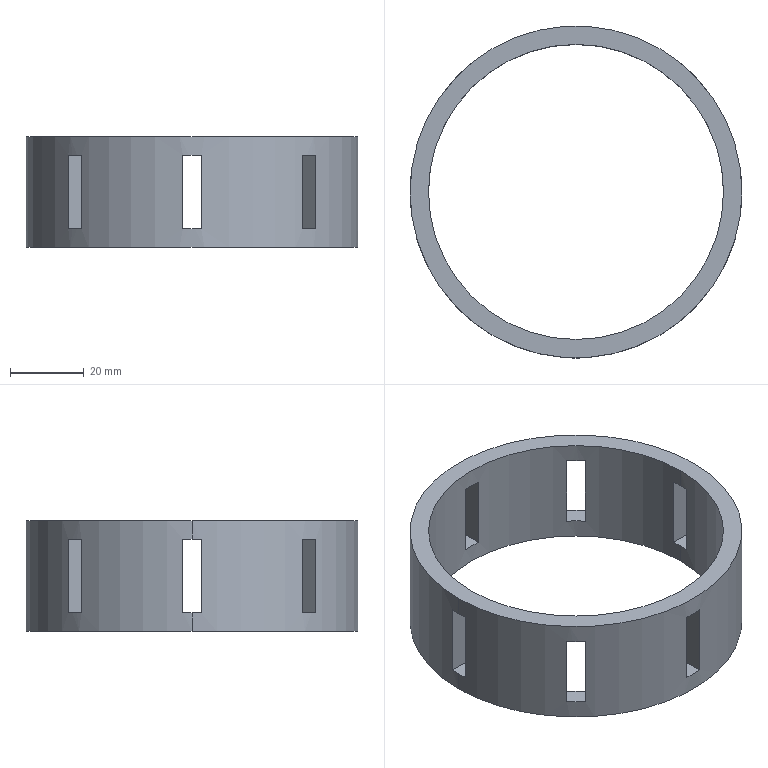Part | SolidWorks | features CirPattern 1, Cut 1, Extrusion 1 | 1 solid | 38 faces | box 90 x 90 x 30 mm | volume 36053 mm3 | plane 34 | cylinder 4 | commonest cylinder face diameters 80 x2 90 x2
STEP:
#1=CARTESIAN_POINT('',(-597.384,-129.922,25.));
#2=VERTEX_POINT('',#1);
#3=CARTESIAN_POINT('',(-597.384,-129.922,5.));
#4=VERTEX_POINT('',#3);
#5=CARTESIAN_POINT('',(-597.384,-129.922,30.));
#6=DIRECTION('',(0.,0.,-1.));
#7=VECTOR('',#6,1000.);
#8=LINE('',#5,#7);
#9=EDGE_CURVE('',#2,#4,#8,.T.);
#10=ORIENTED_EDGE('',*,*,#9,.F.);
#11=CARTESIAN_POINT('',(-602.384,-129.922,25.));
#12=VERTEX_POINT('',#11);
#13=CARTESIAN_POINT('',(-599.884,-90.,25.));
#14=DIRECTION('',(0.,0.,1.));
#15=DIRECTION('',(1.,0.,0.));
#16=AXIS2_PLACEMENT_3D('',#13,#14,#15);
#17=CIRCLE('',#16,40.);
#18=EDGE_CURVE('',#12,#2,#17,.T.);
#19=ORIENTED_EDGE('',*,*,#18,.F.);
#20=CARTESIAN_POINT('',(-602.384,-129.922,5.));
#21=VERTEX_POINT('',#20);
#22=CARTESIAN_POINT('',(-602.384,-129.922,30.));
#23=DIRECTION('',(0.,0.,1.));
#24=VECTOR('',#23,1000.);
#25=LINE('',#22,#24);
#26=EDGE_CURVE('',#21,#12,#25,.T.);
#27=ORIENTED_EDGE('',*,*,#26,.F.);
#28=CARTESIAN_POINT('',(-599.884,-90.,5.));
#29=DIRECTION('',(0.,0.,-1.));
#30=DIRECTION('',(-1.,0.,0.));
#31=AXIS2_PLACEMENT_3D('',#28,#29,#30);
#32=CIRCLE('',#31,40.);
#33=EDGE_CURVE('',#4,#21,#32,.T.);
#34=ORIENTED_EDGE('',*,*,#33,.F.);
#35=EDGE_LOOP('',(#10,#19,#27,#34));
#36=FACE_BOUND('',#35,.T.);
#37=CARTESIAN_POINT('',(-629.881,-116.461,5.));
#38=VERTEX_POINT('',#37);
#39=CARTESIAN_POINT('',(-629.881,-116.461,25.));
#40=VERTEX_POINT('',#39);
#41=CARTESIAN_POINT('',(-629.881,-116.461,30.));
#42=DIRECTION('',(0.,0.,1.));
#43=VECTOR('',#42,1000.);
#44=LINE('',#41,#43);
#45=EDGE_CURVE('',#38,#40,#44,.T.);
#46=ORIENTED_EDGE('',*,*,#45,.F.);
#47=CARTESIAN_POINT('',(-626.345,-119.997,5.));
#48=VERTEX_POINT('',#47);
#49=CARTESIAN_POINT('',(-599.884,-90.,5.));
#50=DIRECTION('',(0.,0.,-1.));
#51=DIRECTION('',(-1.,0.,0.));
#52=AXIS2_PLACEMENT_3D('',#49,#50,#51);
#53=CIRCLE('',#52,40.);
#54=EDGE_CURVE('',#48,#38,#53,.T.);
#55=ORIENTED_EDGE('',*,*,#54,.F.);
#56=CARTESIAN_POINT('',(-626.345,-119.997,25.));
#57=VERTEX_POINT('',#56);
#58=CARTESIAN_POINT('',(-626.345,-119.997,30.));
#59=DIRECTION('',(0.,0.,-1.));
#60=VECTOR('',#59,1000.);
#61=LINE('',#58,#60);
#62=EDGE_CURVE('',#57,#48,#61,.T.);
#63=ORIENTED_EDGE('',*,*,#62,.F.);
#64=CARTESIAN_POINT('',(-599.884,-90.,25.));
#65=DIRECTION('',(0.,0.,1.));
#66=DIRECTION('',(1.,0.,0.));
#67=AXIS2_PLACEMENT_3D('',#64,#65,#66);
#68=CIRCLE('',#67,40.);
#69=EDGE_CURVE('',#40,#57,#68,.T.);
#70=ORIENTED_EDGE('',*,*,#69,.F.);
#71=EDGE_LOOP('',(#46,#55,#63,#70));
#72=FACE_BOUND('',#71,.T.);
#73=CARTESIAN_POINT('',(-569.887,-116.461,25.));
#74=VERTEX_POINT('',#73);
#75=CARTESIAN_POINT('',(-569.887,-116.461,5.));
#76=VERTEX_POINT('',#75);
#77=CARTESIAN_POINT('',(-569.887,-116.461,30.));
#78=DIRECTION('',(0.,0.,-1.));
#79=VECTOR('',#78,1000.);
#80=LINE('',#77,#79);
#81=EDGE_CURVE('',#74,#76,#80,.T.);
#82=ORIENTED_EDGE('',*,*,#81,.F.);
#83=CARTESIAN_POINT('',(-573.423,-119.997,25.));
#84=VERTEX_POINT('',#83);
#85=CARTESIAN_POINT('',(-599.884,-90.,25.));
#86=DIRECTION('',(0.,0.,1.));
#87=DIRECTION('',(1.,0.,0.));
#88=AXIS2_PLACEMENT_3D('',#85,#86,#87);
#89=CIRCLE('',#88,40.);
#90=EDGE_CURVE('',#84,#74,#89,.T.);
#91=ORIENTED_EDGE('',*,*,#90,.F.);
#92=CARTESIAN_POINT('',(-573.423,-119.997,5.));
#93=VERTEX_POINT('',#92);
#94=CARTESIAN_POINT('',(-573.423,-119.997,30.));
#95=DIRECTION('',(0.,0.,1.));
#96=VECTOR('',#95,1000.);
#97=LINE('',#94,#96);
#98=EDGE_CURVE('',#93,#84,#97,.T.);
#99=ORIENTED_EDGE('',*,*,#98,.F.);
#100=CARTESIAN_POINT('',(-599.884,-90.,5.));
#101=DIRECTION('',(0.,0.,-1.));
#102=DIRECTION('',(-1.,0.,0.));
#103=AXIS2_PLACEMENT_3D('',#100,#101,#102);
#104=CIRCLE('',#103,40.);
#105=EDGE_CURVE('',#76,#93,#104,.T.);
#106=ORIENTED_EDGE('',*,*,#105,.F.);
#107=EDGE_LOOP('',(#82,#91,#99,#106));
#108=FACE_BOUND('',#107,.T.);
#109=CARTESIAN_POINT('',(-639.884,-90.,30.));
#110=VERTEX_POINT('',#109);
#111=CARTESIAN_POINT('',(-559.884,-90.,30.));
#112=VERTEX_POINT('',#111);
#113=CARTESIAN_POINT('',(-599.884,-90.,30.));
#114=DIRECTION('',(0.,0.,1.));
#115=DIRECTION('',(1.,0.,0.));
#116=AXIS2_PLACEMENT_3D('',#113,#114,#115);
#117=CIRCLE('',#116,40.);
#118=EDGE_CURVE('',#110,#112,#117,.T.);
#119=ORIENTED_EDGE('',*,*,#118,.T.);
#120=CARTESIAN_POINT('',(-559.884,-90.,25.));
#121=VERTEX_POINT('',#120);
#122=CARTESIAN_POINT('',(-559.884,-90.,30.));
#123=DIRECTION('',(0.,0.,-1.));
#124=VECTOR('',#123,1000.);
#125=LINE('',#122,#124);
#126=EDGE_CURVE('',#112,#121,#125,.T.);
#127=ORIENTED_EDGE('',*,*,#126,.T.);
#128=CARTESIAN_POINT('',(-559.962,-92.5,25.));
#129=VERTEX_POINT('',#128);
#130=CARTESIAN_POINT('',(-599.884,-90.,25.));
#131=DIRECTION('',(0.,0.,1.));
#132=DIRECTION('',(1.,0.,0.));
#133=AXIS2_PLACEMENT_3D('',#130,#131,#132);
#134=CIRCLE('',#133,40.);
#135=EDGE_CURVE('',#129,#121,#134,.T.);
#136=ORIENTED_EDGE('',*,*,#135,.F.);
#137=CARTESIAN_POINT('',(-559.962,-92.5,5.));
#138=VERTEX_POINT('',#137);
#139=CARTESIAN_POINT('',(-559.962,-92.5,30.));
#140=DIRECTION('',(0.,0.,1.));
#141=VECTOR('',#140,1000.);
#142=LINE('',#139,#141);
#143=EDGE_CURVE('',#138,#129,#142,.T.);
#144=ORIENTED_EDGE('',*,*,#143,.F.);
#145=CARTESIAN_POINT('',(-559.884,-90.,5.));
#146=VERTEX_POINT('',#145);
#147=CARTESIAN_POINT('',(-599.884,-90.,5.));
#148=DIRECTION('',(0.,0.,-1.));
#149=DIRECTION('',(-1.,0.,0.));
#150=AXIS2_PLACEMENT_3D('',#147,#148,#149);
#151=CIRCLE('',#150,40.);
#152=EDGE_CURVE('',#146,#138,#151,.T.);
#153=ORIENTED_EDGE('',*,*,#152,.F.);
#154=CARTESIAN_POINT('',(-559.884,-90.,0.));
#155=VERTEX_POINT('',#154);
#156=CARTESIAN_POINT('',(-559.884,-90.,30.));
#157=DIRECTION('',(0.,0.,-1.));
#158=VECTOR('',#157,1000.);
#159=LINE('',#156,#158);
#160=EDGE_CURVE('',#146,#155,#159,.T.);
#161=ORIENTED_EDGE('',*,*,#160,.T.);
#162=CARTESIAN_POINT('',(-639.884,-90.,0.));
#163=VERTEX_POINT('',#162);
#164=CARTESIAN_POINT('',(-599.884,-90.,0.));
#165=DIRECTION('',(0.,0.,1.));
#166=DIRECTION('',(1.,0.,0.));
#167=AXIS2_PLACEMENT_3D('',#164,#165,#166);
#168=CIRCLE('',#167,40.);
#169=EDGE_CURVE('',#163,#155,#168,.T.);
#170=ORIENTED_EDGE('',*,*,#169,.F.);
#171=CARTESIAN_POINT('',(-639.884,-90.,5.));
#172=VERTEX_POINT('',#171);
#173=CARTESIAN_POINT('',(-639.884,-90.,30.));
#174=DIRECTION('',(0.,0.,-1.));
#175=VECTOR('',#174,1000.);
#176=LINE('',#173,#175);
#177=EDGE_CURVE('',#172,#163,#176,.T.);
#178=ORIENTED_EDGE('',*,*,#177,.F.);
#179=CARTESIAN_POINT('',(-639.806,-92.5,5.));
#180=VERTEX_POINT('',#179);
#181=CARTESIAN_POINT('',(-599.884,-90.,5.));
#182=DIRECTION('',(0.,0.,-1.));
#183=DIRECTION('',(-1.,0.,0.));
#184=AXIS2_PLACEMENT_3D('',#181,#182,#183);
#185=CIRCLE('',#184,40.);
#186=EDGE_CURVE('',#180,#172,#185,.T.);
#187=ORIENTED_EDGE('',*,*,#186,.F.);
#188=CARTESIAN_POINT('',(-639.806,-92.5,25.));
#189=VERTEX_POINT('',#188);
#190=CARTESIAN_POINT('',(-639.806,-92.5,30.));
#191=DIRECTION('',(0.,0.,-1.));
#192=VECTOR('',#191,1000.);
#193=LINE('',#190,#192);
#194=EDGE_CURVE('',#189,#180,#193,.T.);
#195=ORIENTED_EDGE('',*,*,#194,.F.);
#196=CARTESIAN_POINT('',(-639.884,-90.,25.));
#197=VERTEX_POINT('',#196);
#198=CARTESIAN_POINT('',(-599.884,-90.,25.));
#199=DIRECTION('',(0.,0.,1.));
#200=DIRECTION('',(1.,0.,0.));
#201=AXIS2_PLACEMENT_3D('',#198,#199,#200);
#202=CIRCLE('',#201,40.);
#203=EDGE_CURVE('',#197,#189,#202,.T.);
#204=ORIENTED_EDGE('',*,*,#203,.F.);
#205=CARTESIAN_POINT('',(-639.884,-90.,30.));
#206=DIRECTION('',(0.,0.,-1.));
#207=VECTOR('',#206,1000.);
#208=LINE('',#205,#207);
#209=EDGE_CURVE('',#110,#197,#208,.T.);
#210=ORIENTED_EDGE('',*,*,#209,.F.);
#211=EDGE_LOOP('',(#119,#127,#136,#144,#153,#161,#170,#178,#187,#195,#204,#210));
#212=FACE_OUTER_BOUND('',#211,.T.);
#213=CARTESIAN_POINT('',(-599.884,-90.,30.));
#214=DIRECTION('',(0.,0.,-1.));
#215=DIRECTION('',(-1.,0.,0.));
#216=AXIS2_PLACEMENT_3D('',#213,#214,#215);
#217=CYLINDRICAL_SURFACE('',#216,40.);
#218=ADVANCED_FACE('',(#36,#72,#108,#212),#217,.F.);
#219=CARTESIAN_POINT('',(-602.384,-45.069,5.));
#220=VERTEX_POINT('',#219);
#221=CARTESIAN_POINT('',(-597.384,-45.069,5.));
#222=VERTEX_POINT('',#221);
#223=CARTESIAN_POINT('',(-599.884,-90.,5.));
#224=DIRECTION('',(0.,0.,-1.));
#225=DIRECTION('',(-1.,0.,0.));
#226=AXIS2_PLACEMENT_3D('',#223,#224,#225);
#227=CIRCLE('',#226,45.);
#228=EDGE_CURVE('',#220,#222,#227,.T.);
#229=ORIENTED_EDGE('',*,*,#228,.T.);
#230=CARTESIAN_POINT('',(-597.384,-45.069,25.));
#231=VERTEX_POINT('',#230);
#232=CARTESIAN_POINT('',(-597.384,-45.069,30.));
#233=DIRECTION('',(0.,0.,1.));
#234=VECTOR('',#233,1000.);
#235=LINE('',#232,#234);
#236=EDGE_CURVE('',#222,#231,#235,.T.);
#237=ORIENTED_EDGE('',*,*,#236,.T.);
#238=CARTESIAN_POINT('',(-602.384,-45.069,25.));
#239=VERTEX_POINT('',#238);
#240=CARTESIAN_POINT('',(-599.884,-90.,25.));
#241=DIRECTION('',(0.,0.,1.));
#242=DIRECTION('',(1.,0.,0.));
#243=AXIS2_PLACEMENT_3D('',#240,#241,#242);
#244=CIRCLE('',#243,45.);
#245=EDGE_CURVE('',#231,#239,#244,.T.);
#246=ORIENTED_EDGE('',*,*,#245,.T.);
#247=CARTESIAN_POINT('',(-602.384,-45.069,30.));
#248=DIRECTION('',(0.,0.,-1.));
#249=VECTOR('',#248,1000.);
#250=LINE('',#247,#249);
#251=EDGE_CURVE('',#239,#220,#250,.T.);
#252=ORIENTED_EDGE('',*,*,#251,.T.);
#253=EDGE_LOOP('',(#229,#237,#246,#252));
#254=FACE_BOUND('',#253,.T.);
#255=CARTESIAN_POINT('',(-566.346,-59.997,25.));
#256=VERTEX_POINT('',#255);
#257=CARTESIAN_POINT('',(-569.881,-56.462,25.));
#258=VERTEX_POINT('',#257);
#259=CARTESIAN_POINT('',(-599.884,-90.,25.));
#260=DIRECTION('',(0.,0.,1.));
#261=DIRECTION('',(1.,0.,0.));
#262=AXIS2_PLACEMENT_3D('',#259,#260,#261);
#263=CIRCLE('',#262,45.);
#264=EDGE_CURVE('',#256,#258,#263,.T.);
#265=ORIENTED_EDGE('',*,*,#264,.T.);
#266=CARTESIAN_POINT('',(-569.881,-56.462,5.));
#267=VERTEX_POINT('',#266);
#268=CARTESIAN_POINT('',(-569.881,-56.462,30.));
#269=DIRECTION('',(0.,0.,-1.));
#270=VECTOR('',#269,1000.);
#271=LINE('',#268,#270);
#272=EDGE_CURVE('',#258,#267,#271,.T.);
#273=ORIENTED_EDGE('',*,*,#272,.T.);
#274=CARTESIAN_POINT('',(-566.346,-59.997,5.));
#275=VERTEX_POINT('',#274);
#276=CARTESIAN_POINT('',(-599.884,-90.,5.));
#277=DIRECTION('',(0.,0.,-1.));
#278=DIRECTION('',(-1.,0.,0.));
#279=AXIS2_PLACEMENT_3D('',#276,#277,#278);
#280=CIRCLE('',#279,45.);
#281=EDGE_CURVE('',#267,#275,#280,.T.);
#282=ORIENTED_EDGE('',*,*,#281,.T.);
#283=CARTESIAN_POINT('',(-566.346,-59.997,30.));
#284=DIRECTION('',(0.,0.,1.));
#285=VECTOR('',#284,1000.);
#286=LINE('',#283,#285);
#287=EDGE_CURVE('',#275,#256,#286,.T.);
#288=ORIENTED_EDGE('',*,*,#287,.T.);
#289=EDGE_LOOP('',(#265,#273,#282,#288));
#290=FACE_BOUND('',#289,.T.);
#291=CARTESIAN_POINT('',(-629.887,-56.462,5.));
#292=VERTEX_POINT('',#291);
#293=CARTESIAN_POINT('',(-629.887,-56.462,25.));
#294=VERTEX_POINT('',#293);
#295=CARTESIAN_POINT('',(-629.887,-56.462,30.));
#296=DIRECTION('',(0.,0.,1.));
#297=VECTOR('',#296,1000.);
#298=LINE('',#295,#297);
#299=EDGE_CURVE('',#292,#294,#298,.T.);
#300=ORIENTED_EDGE('',*,*,#299,.T.);
#301=CARTESIAN_POINT('',(-633.423,-59.997,25.));
#302=VERTEX_POINT('',#301);
#303=CARTESIAN_POINT('',(-599.884,-90.,25.));
#304=DIRECTION('',(0.,0.,1.));
#305=DIRECTION('',(1.,0.,0.));
#306=AXIS2_PLACEMENT_3D('',#303,#304,#305);
#307=CIRCLE('',#306,45.);
#308=EDGE_CURVE('',#294,#302,#307,.T.);
#309=ORIENTED_EDGE('',*,*,#308,.T.);
#310=CARTESIAN_POINT('',(-633.423,-59.997,5.));
#311=VERTEX_POINT('',#310);
#312=CARTESIAN_POINT('',(-633.423,-59.997,30.));
#313=DIRECTION('',(0.,0.,-1.));
#314=VECTOR('',#313,1000.);
#315=LINE('',#312,#314);
#316=EDGE_CURVE('',#302,#311,#315,.T.);
#317=ORIENTED_EDGE('',*,*,#316,.T.);
#318=CARTESIAN_POINT('',(-599.884,-90.,5.));
#319=DIRECTION('',(0.,0.,-1.));
#320=DIRECTION('',(-1.,0.,0.));
#321=AXIS2_PLACEMENT_3D('',#318,#319,#320);
#322=CIRCLE('',#321,45.);
#323=EDGE_CURVE('',#311,#292,#322,.T.);
#324=ORIENTED_EDGE('',*,*,#323,.T.);
#325=EDGE_LOOP('',(#300,#309,#317,#324));
#326=FACE_BOUND('',#325,.T.);
#327=CARTESIAN_POINT('',(-554.884,-90.,30.));
#328=VERTEX_POINT('',#327);
#329=CARTESIAN_POINT('',(-644.884,-90.,30.));
#330=VERTEX_POINT('',#329);
#331=CARTESIAN_POINT('',(-599.884,-90.,30.));
#332=DIRECTION('',(0.,0.,1.));
#333=DIRECTION('',(1.,0.,0.));
#334=AXIS2_PLACEMENT_3D('',#331,#332,#333);
#335=CIRCLE('',#334,45.);
#336=EDGE_CURVE('',#328,#330,#335,.T.);
#337=ORIENTED_EDGE('',*,*,#336,.F.);
#338=CARTESIAN_POINT('',(-554.884,-90.,25.));
#339=VERTEX_POINT('',#338);
#340=CARTESIAN_POINT('',(-554.884,-90.,30.));
#341=DIRECTION('',(0.,0.,-1.));
#342=VECTOR('',#341,1000.);
#343=LINE('',#340,#342);
#344=EDGE_CURVE('',#328,#339,#343,.T.);
#345=ORIENTED_EDGE('',*,*,#344,.T.);
#346=CARTESIAN_POINT('',(-554.954,-87.5,25.));
#347=VERTEX_POINT('',#346);
#348=CARTESIAN_POINT('',(-599.884,-90.,25.));
#349=DIRECTION('',(0.,0.,1.));
#350=DIRECTION('',(1.,0.,0.));
#351=AXIS2_PLACEMENT_3D('',#348,#349,#350);
#352=CIRCLE('',#351,45.);
#353=EDGE_CURVE('',#339,#347,#352,.T.);
#354=ORIENTED_EDGE('',*,*,#353,.T.);
#355=CARTESIAN_POINT('',(-554.954,-87.5,5.));
#356=VERTEX_POINT('',#355);
#357=CARTESIAN_POINT('',(-554.954,-87.5,30.));
#358=DIRECTION('',(0.,0.,-1.));
#359=VECTOR('',#358,1000.);
#360=LINE('',#357,#359);
#361=EDGE_CURVE('',#347,#356,#360,.T.);
#362=ORIENTED_EDGE('',*,*,#361,.T.);
#363=CARTESIAN_POINT('',(-554.884,-90.,5.));
#364=VERTEX_POINT('',#363);
#365=CARTESIAN_POINT('',(-599.884,-90.,5.));
#366=DIRECTION('',(0.,0.,-1.));
#367=DIRECTION('',(-1.,0.,0.));
#368=AXIS2_PLACEMENT_3D('',#365,#366,#367);
#369=CIRCLE('',#368,45.);
#370=EDGE_CURVE('',#356,#364,#369,.T.);
#371=ORIENTED_EDGE('',*,*,#370,.T.);
#372=CARTESIAN_POINT('',(-554.884,-90.,0.));
#373=VERTEX_POINT('',#372);
#374=CARTESIAN_POINT('',(-554.884,-90.,30.));
#375=DIRECTION('',(0.,0.,-1.));
#376=VECTOR('',#375,1000.);
#377=LINE('',#374,#376);
#378=EDGE_CURVE('',#364,#373,#377,.T.);
#379=ORIENTED_EDGE('',*,*,#378,.T.);
#380=CARTESIAN_POINT('',(-644.884,-90.,0.));
#381=VERTEX_POINT('',#380);
#382=CARTESIAN_POINT('',(-599.884,-90.,0.));
#383=DIRECTION('',(0.,0.,1.));
#384=DIRECTION('',(1.,0.,0.));
#385=AXIS2_PLACEMENT_3D('',#382,#383,#384);
#386=CIRCLE('',#385,45.);
#387=EDGE_CURVE('',#373,#381,#386,.T.);
#388=ORIENTED_EDGE('',*,*,#387,.T.);
#389=CARTESIAN_POINT('',(-644.884,-90.,5.));
#390=VERTEX_POINT('',#389);
#391=CARTESIAN_POINT('',(-644.884,-90.,30.));
#392=DIRECTION('',(0.,0.,-1.));
#393=VECTOR('',#392,1000.);
#394=LINE('',#391,#393);
#395=EDGE_CURVE('',#390,#381,#394,.T.);
#396=ORIENTED_EDGE('',*,*,#395,.F.);
#397=CARTESIAN_POINT('',(-644.815,-87.5,5.));
#398=VERTEX_POINT('',#397);
#399=CARTESIAN_POINT('',(-599.884,-90.,5.));
#400=DIRECTION('',(0.,0.,-1.));
#401=DIRECTION('',(-1.,0.,0.));
#402=AXIS2_PLACEMENT_3D('',#399,#400,#401);
#403=CIRCLE('',#402,45.);
#404=EDGE_CURVE('',#390,#398,#403,.T.);
#405=ORIENTED_EDGE('',*,*,#404,.T.);
#406=CARTESIAN_POINT('',(-644.815,-87.5,25.));
#407=VERTEX_POINT('',#406);
#408=CARTESIAN_POINT('',(-644.815,-87.5,30.));
#409=DIRECTION('',(0.,0.,1.));
#410=VECTOR('',#409,1000.);
#411=LINE('',#408,#410);
#412=EDGE_CURVE('',#398,#407,#411,.T.);
#413=ORIENTED_EDGE('',*,*,#412,.T.);
#414=CARTESIAN_POINT('',(-644.884,-90.,25.));
#415=VERTEX_POINT('',#414);
#416=CARTESIAN_POINT('',(-599.884,-90.,25.));
#417=DIRECTION('',(0.,0.,1.));
#418=DIRECTION('',(1.,0.,0.));
#419=AXIS2_PLACEMENT_3D('',#416,#417,#418);
#420=CIRCLE('',#419,45.);
#421=EDGE_CURVE('',#407,#415,#420,.T.);
#422=ORIENTED_EDGE('',*,*,#421,.T.);
#423=CARTESIAN_POINT('',(-644.884,-90.,30.));
#424=DIRECTION('',(0.,0.,-1.));
#425=VECTOR('',#424,1000.);
#426=LINE('',#423,#425);
#427=EDGE_CURVE('',#330,#415,#426,.T.);
#428=ORIENTED_EDGE('',*,*,#427,.F.);
#429=EDGE_LOOP('',(#337,#345,#354,#362,#371,#379,#388,#396,#405,#413,#422,#428));
#430=FACE_OUTER_BOUND('',#429,.T.);
#431=CARTESIAN_POINT('',(-599.884,-90.,30.));
#432=DIRECTION('',(0.,0.,-1.));
#433=DIRECTION('',(-1.,0.,0.));
#434=AXIS2_PLACEMENT_3D('',#431,#432,#433);
#435=CYLINDRICAL_SURFACE('',#434,45.);
#436=ADVANCED_FACE('',(#254,#290,#326,#430),#435,.T.);
#437=CARTESIAN_POINT('',(-599.884,-90.,30.));
#438=DIRECTION('',(0.,0.,1.));
#439=DIRECTION('',(1.,0.,0.));
#440=AXIS2_PLACEMENT_3D('',#437,#438,#439);
#441=CIRCLE('',#440,45.);
#442=EDGE_CURVE('',#330,#328,#441,.T.);
#443=ORIENTED_EDGE('',*,*,#442,.T.);
#444=ORIENTED_EDGE('',*,*,#336,.T.);
#445=EDGE_LOOP('',(#443,#444));
#446=FACE_OUTER_BOUND('',#445,.T.);
#447=ORIENTED_EDGE('',*,*,#118,.F.);
#448=CARTESIAN_POINT('',(-599.884,-90.,30.));
#449=DIRECTION('',(0.,0.,1.));
#450=DIRECTION('',(1.,0.,0.));
#451=AXIS2_PLACEMENT_3D('',#448,#449,#450);
#452=CIRCLE('',#451,40.);
#453=EDGE_CURVE('',#112,#110,#452,.T.);
#454=ORIENTED_EDGE('',*,*,#453,.F.);
#455=EDGE_LOOP('',(#447,#454));
#456=FACE_BOUND('',#455,.T.);
#457=CARTESIAN_POINT('',(-599.884,-90.,30.));
#458=DIRECTION('',(0.,0.,1.));
#459=DIRECTION('',(1.,0.,0.));
#460=AXIS2_PLACEMENT_3D('',#457,#458,#459);
#461=PLANE('',#460);
#462=ADVANCED_FACE('',(#446,#456),#461,.T.);
#463=CARTESIAN_POINT('',(-599.884,-90.,0.));
#464=DIRECTION('',(0.,0.,1.));
#465=DIRECTION('',(1.,0.,0.));
#466=AXIS2_PLACEMENT_3D('',#463,#464,#465);
#467=CIRCLE('',#466,45.);
#468=EDGE_CURVE('',#381,#373,#467,.T.);
#469=ORIENTED_EDGE('',*,*,#468,.F.);
#470=ORIENTED_EDGE('',*,*,#387,.F.);
#471=EDGE_LOOP('',(#469,#470));
#472=FACE_OUTER_BOUND('',#471,.T.);
#473=ORIENTED_EDGE('',*,*,#169,.T.);
#474=CARTESIAN_POINT('',(-599.884,-90.,0.));
#475=DIRECTION('',(0.,0.,1.));
#476=DIRECTION('',(1.,0.,0.));
#477=AXIS2_PLACEMENT_3D('',#474,#475,#476);
#478=CIRCLE('',#477,40.);
#479=EDGE_CURVE('',#155,#163,#478,.T.);
#480=ORIENTED_EDGE('',*,*,#479,.T.);
#481=EDGE_LOOP('',(#473,#480));
#482=FACE_BOUND('',#481,.T.);
#483=CARTESIAN_POINT('',(-599.884,-90.,0.));
#484=DIRECTION('',(0.,0.,1.));
#485=DIRECTION('',(1.,0.,0.));
#486=AXIS2_PLACEMENT_3D('',#483,#484,#485);
#487=PLANE('',#486);
#488=ADVANCED_FACE('',(#472,#482),#487,.F.);
#489=ORIENTED_EDGE('',*,*,#344,.F.);
#490=ORIENTED_EDGE('',*,*,#442,.F.);
#491=ORIENTED_EDGE('',*,*,#427,.T.);
#492=CARTESIAN_POINT('',(-644.815,-92.5,25.));
#493=VERTEX_POINT('',#492);
#494=CARTESIAN_POINT('',(-599.884,-90.,25.));
#495=DIRECTION('',(0.,0.,1.));
#496=DIRECTION('',(1.,0.,0.));
#497=AXIS2_PLACEMENT_3D('',#494,#495,#496);
#498=CIRCLE('',#497,45.);
#499=EDGE_CURVE('',#415,#493,#498,.T.);
#500=ORIENTED_EDGE('',*,*,#499,.T.);
#501=CARTESIAN_POINT('',(-644.815,-92.5,5.));
#502=VERTEX_POINT('',#501);
#503=CARTESIAN_POINT('',(-644.815,-92.5,30.));
#504=DIRECTION('',(0.,0.,-1.));
#505=VECTOR('',#504,1000.);
#506=LINE('',#503,#505);
#507=EDGE_CURVE('',#493,#502,#506,.T.);
#508=ORIENTED_EDGE('',*,*,#507,.T.);
#509=CARTESIAN_POINT('',(-599.884,-90.,5.));
#510=DIRECTION('',(0.,0.,-1.));
#511=DIRECTION('',(-1.,0.,0.));
#512=AXIS2_PLACEMENT_3D('',#509,#510,#511);
#513=CIRCLE('',#512,45.);
#514=EDGE_CURVE('',#502,#390,#513,.T.);
#515=ORIENTED_EDGE('',*,*,#514,.T.);
#516=ORIENTED_EDGE('',*,*,#395,.T.);
#517=ORIENTED_EDGE('',*,*,#468,.T.);
#518=ORIENTED_EDGE('',*,*,#378,.F.);
#519=CARTESIAN_POINT('',(-554.954,-92.5,5.));
#520=VERTEX_POINT('',#519);
#521=CARTESIAN_POINT('',(-599.884,-90.,5.));
#522=DIRECTION('',(0.,0.,-1.));
#523=DIRECTION('',(-1.,0.,0.));
#524=AXIS2_PLACEMENT_3D('',#521,#522,#523);
#525=CIRCLE('',#524,45.);
#526=EDGE_CURVE('',#364,#520,#525,.T.);
#527=ORIENTED_EDGE('',*,*,#526,.T.);
#528=CARTESIAN_POINT('',(-554.954,-92.5,25.));
#529=VERTEX_POINT('',#528);
#530=CARTESIAN_POINT('',(-554.954,-92.5,30.));
#531=DIRECTION('',(0.,0.,1.));
#532=VECTOR('',#531,1000.);
#533=LINE('',#530,#532);
#534=EDGE_CURVE('',#520,#529,#533,.T.);
#535=ORIENTED_EDGE('',*,*,#534,.T.);
#536=CARTESIAN_POINT('',(-599.884,-90.,25.));
#537=DIRECTION('',(0.,0.,1.));
#538=DIRECTION('',(1.,0.,0.));
#539=AXIS2_PLACEMENT_3D('',#536,#537,#538);
#540=CIRCLE('',#539,45.);
#541=EDGE_CURVE('',#529,#339,#540,.T.);
#542=ORIENTED_EDGE('',*,*,#541,.T.);
#543=EDGE_LOOP('',(#489,#490,#491,#500,#508,#515,#516,#517,#518,#527,#535,#542));
#544=FACE_OUTER_BOUND('',#543,.T.);
#545=CARTESIAN_POINT('',(-569.881,-123.538,25.));
#546=VERTEX_POINT('',#545);
#547=CARTESIAN_POINT('',(-566.346,-120.003,25.));
#548=VERTEX_POINT('',#547);
#549=CARTESIAN_POINT('',(-599.884,-90.,25.));
#550=DIRECTION('',(0.,0.,1.));
#551=DIRECTION('',(1.,0.,0.));
#552=AXIS2_PLACEMENT_3D('',#549,#550,#551);
#553=CIRCLE('',#552,45.);
#554=EDGE_CURVE('',#546,#548,#553,.T.);
#555=ORIENTED_EDGE('',*,*,#554,.T.);
#556=CARTESIAN_POINT('',(-566.346,-120.003,5.));
#557=VERTEX_POINT('',#556);
#558=CARTESIAN_POINT('',(-566.346,-120.003,30.));
#559=DIRECTION('',(0.,0.,-1.));
#560=VECTOR('',#559,1000.);
#561=LINE('',#558,#560);
#562=EDGE_CURVE('',#548,#557,#561,.T.);
#563=ORIENTED_EDGE('',*,*,#562,.T.);
#564=CARTESIAN_POINT('',(-569.881,-123.538,5.));
#565=VERTEX_POINT('',#564);
#566=CARTESIAN_POINT('',(-599.884,-90.,5.));
#567=DIRECTION('',(0.,0.,-1.));
#568=DIRECTION('',(-1.,0.,0.));
#569=AXIS2_PLACEMENT_3D('',#566,#567,#568);
#570=CIRCLE('',#569,45.);
#571=EDGE_CURVE('',#557,#565,#570,.T.);
#572=ORIENTED_EDGE('',*,*,#571,.T.);
#573=CARTESIAN_POINT('',(-569.881,-123.538,30.));
#574=DIRECTION('',(0.,0.,1.));
#575=VECTOR('',#574,1000.);
#576=LINE('',#573,#575);
#577=EDGE_CURVE('',#565,#546,#576,.T.);
#578=ORIENTED_EDGE('',*,*,#577,.T.);
#579=EDGE_LOOP('',(#555,#563,#572,#578));
#580=FACE_BOUND('',#579,.T.);
#581=CARTESIAN_POINT('',(-629.887,-123.538,5.));
#582=VERTEX_POINT('',#581);
#583=CARTESIAN_POINT('',(-633.423,-120.003,5.));
#584=VERTEX_POINT('',#583);
#585=CARTESIAN_POINT('',(-599.884,-90.,5.));
#586=DIRECTION('',(0.,0.,-1.));
#587=DIRECTION('',(-1.,0.,0.));
#588=AXIS2_PLACEMENT_3D('',#585,#586,#587);
#589=CIRCLE('',#588,45.);
#590=EDGE_CURVE('',#582,#584,#589,.T.);
#591=ORIENTED_EDGE('',*,*,#590,.T.);
#592=CARTESIAN_POINT('',(-633.423,-120.003,25.));
#593=VERTEX_POINT('',#592);
#594=CARTESIAN_POINT('',(-633.423,-120.003,30.));
#595=DIRECTION('',(0.,0.,1.));
#596=VECTOR('',#595,1000.);
#597=LINE('',#594,#596);
#598=EDGE_CURVE('',#584,#593,#597,.T.);
#599=ORIENTED_EDGE('',*,*,#598,.T.);
#600=CARTESIAN_POINT('',(-629.887,-123.538,25.));
#601=VERTEX_POINT('',#600);
#602=CARTESIAN_POINT('',(-599.884,-90.,25.));
#603=DIRECTION('',(0.,0.,1.));
#604=DIRECTION('',(1.,0.,0.));
#605=AXIS2_PLACEMENT_3D('',#602,#603,#604);
#606=CIRCLE('',#605,45.);
#607=EDGE_CURVE('',#593,#601,#606,.T.);
#608=ORIENTED_EDGE('',*,*,#607,.T.);
#609=CARTESIAN_POINT('',(-629.887,-123.538,30.));
#610=DIRECTION('',(0.,0.,-1.));
#611=VECTOR('',#610,1000.);
#612=LINE('',#609,#611);
#613=EDGE_CURVE('',#601,#582,#612,.T.);
#614=ORIENTED_EDGE('',*,*,#613,.T.);
#615=EDGE_LOOP('',(#591,#599,#608,#614));
#616=FACE_BOUND('',#615,.T.);
#617=CARTESIAN_POINT('',(-597.384,-134.931,25.));
#618=VERTEX_POINT('',#617);
#619=CARTESIAN_POINT('',(-597.384,-134.931,5.));
#620=VERTEX_POINT('',#619);
#621=CARTESIAN_POINT('',(-597.384,-134.931,30.));
#622=DIRECTION('',(0.,0.,-1.));
#623=VECTOR('',#622,1000.);
#624=LINE('',#621,#623);
#625=EDGE_CURVE('',#618,#620,#624,.T.);
#626=ORIENTED_EDGE('',*,*,#625,.T.);
#627=CARTESIAN_POINT('',(-602.384,-134.931,5.));
#628=VERTEX_POINT('',#627);
#629=CARTESIAN_POINT('',(-599.884,-90.,5.));
#630=DIRECTION('',(0.,0.,-1.));
#631=DIRECTION('',(-1.,0.,0.));
#632=AXIS2_PLACEMENT_3D('',#629,#630,#631);
#633=CIRCLE('',#632,45.);
#634=EDGE_CURVE('',#620,#628,#633,.T.);
#635=ORIENTED_EDGE('',*,*,#634,.T.);
#636=CARTESIAN_POINT('',(-602.384,-134.931,25.));
#637=VERTEX_POINT('',#636);
#638=CARTESIAN_POINT('',(-602.384,-134.931,30.));
#639=DIRECTION('',(0.,0.,1.));
#640=VECTOR('',#639,1000.);
#641=LINE('',#638,#640);
#642=EDGE_CURVE('',#628,#637,#641,.T.);
#643=ORIENTED_EDGE('',*,*,#642,.T.);
#644=CARTESIAN_POINT('',(-599.884,-90.,25.));
#645=DIRECTION('',(0.,0.,1.));
#646=DIRECTION('',(1.,0.,0.));
#647=AXIS2_PLACEMENT_3D('',#644,#645,#646);
#648=CIRCLE('',#647,45.);
#649=EDGE_CURVE('',#637,#618,#648,.T.);
#650=ORIENTED_EDGE('',*,*,#649,.T.);
#651=EDGE_LOOP('',(#626,#635,#643,#650));
#652=FACE_BOUND('',#651,.T.);
#653=CARTESIAN_POINT('',(-599.884,-90.,30.));
#654=DIRECTION('',(0.,0.,-1.));
#655=DIRECTION('',(-1.,0.,0.));
#656=AXIS2_PLACEMENT_3D('',#653,#654,#655);
#657=CYLINDRICAL_SURFACE('',#656,45.);
#658=ADVANCED_FACE('',(#544,#580,#616,#652),#657,.T.);
#659=ORIENTED_EDGE('',*,*,#126,.F.);
#660=ORIENTED_EDGE('',*,*,#453,.T.);
#661=ORIENTED_EDGE('',*,*,#209,.T.);
#662=CARTESIAN_POINT('',(-639.806,-87.5,25.));
#663=VERTEX_POINT('',#662);
#664=CARTESIAN_POINT('',(-599.884,-90.,25.));
#665=DIRECTION('',(0.,0.,1.));
#666=DIRECTION('',(1.,0.,0.));
#667=AXIS2_PLACEMENT_3D('',#664,#665,#666);
#668=CIRCLE('',#667,40.);
#669=EDGE_CURVE('',#663,#197,#668,.T.);
#670=ORIENTED_EDGE('',*,*,#669,.F.);
#671=CARTESIAN_POINT('',(-639.806,-87.5,5.));
#672=VERTEX_POINT('',#671);
#673=CARTESIAN_POINT('',(-639.806,-87.5,30.));
#674=DIRECTION('',(0.,0.,1.));
#675=VECTOR('',#674,1000.);
#676=LINE('',#673,#675);
#677=EDGE_CURVE('',#672,#663,#676,.T.);
#678=ORIENTED_EDGE('',*,*,#677,.F.);
#679=CARTESIAN_POINT('',(-599.884,-90.,5.));
#680=DIRECTION('',(0.,0.,-1.));
#681=DIRECTION('',(-1.,0.,0.));
#682=AXIS2_PLACEMENT_3D('',#679,#680,#681);
#683=CIRCLE('',#682,40.);
#684=EDGE_CURVE('',#172,#672,#683,.T.);
#685=ORIENTED_EDGE('',*,*,#684,.F.);
#686=ORIENTED_EDGE('',*,*,#177,.T.);
#687=ORIENTED_EDGE('',*,*,#479,.F.);
#688=ORIENTED_EDGE('',*,*,#160,.F.);
#689=CARTESIAN_POINT('',(-559.962,-87.5,5.));
#690=VERTEX_POINT('',#689);
#691=CARTESIAN_POINT('',(-599.884,-90.,5.));
#692=DIRECTION('',(0.,0.,-1.));
#693=DIRECTION('',(-1.,0.,0.));
#694=AXIS2_PLACEMENT_3D('',#691,#692,#693);
#695=CIRCLE('',#694,40.);
#696=EDGE_CURVE('',#690,#146,#695,.T.);
#697=ORIENTED_EDGE('',*,*,#696,.F.);
#698=CARTESIAN_POINT('',(-559.962,-87.5,25.));
#699=VERTEX_POINT('',#698);
#700=CARTESIAN_POINT('',(-559.962,-87.5,30.));
#701=DIRECTION('',(0.,0.,-1.));
#702=VECTOR('',#701,1000.);
#703=LINE('',#700,#702);
#704=EDGE_CURVE('',#699,#690,#703,.T.);
#705=ORIENTED_EDGE('',*,*,#704,.F.);
#706=CARTESIAN_POINT('',(-599.884,-90.,25.));
#707=DIRECTION('',(0.,0.,1.));
#708=DIRECTION('',(1.,0.,0.));
#709=AXIS2_PLACEMENT_3D('',#706,#707,#708);
#710=CIRCLE('',#709,40.);
#711=EDGE_CURVE('',#121,#699,#710,.T.);
#712=ORIENTED_EDGE('',*,*,#711,.F.);
#713=EDGE_LOOP('',(#659,#660,#661,#670,#678,#685,#686,#687,#688,#697,#705,#712));
#714=FACE_OUTER_BOUND('',#713,.T.);
#715=CARTESIAN_POINT('',(-626.345,-60.003,25.));
#716=VERTEX_POINT('',#715);
#717=CARTESIAN_POINT('',(-629.881,-63.539,25.));
#718=VERTEX_POINT('',#717);
#719=CARTESIAN_POINT('',(-599.884,-90.,25.));
#720=DIRECTION('',(0.,0.,1.));
#721=DIRECTION('',(1.,0.,0.));
#722=AXIS2_PLACEMENT_3D('',#719,#720,#721);
#723=CIRCLE('',#722,40.);
#724=EDGE_CURVE('',#716,#718,#723,.T.);
#725=ORIENTED_EDGE('',*,*,#724,.F.);
#726=CARTESIAN_POINT('',(-626.345,-60.003,5.));
#727=VERTEX_POINT('',#726);
#728=CARTESIAN_POINT('',(-626.345,-60.003,30.));
#729=DIRECTION('',(0.,0.,1.));
#730=VECTOR('',#729,1000.);
#731=LINE('',#728,#730);
#732=EDGE_CURVE('',#727,#716,#731,.T.);
#733=ORIENTED_EDGE('',*,*,#732,.F.);
#734=CARTESIAN_POINT('',(-629.881,-63.539,5.));
#735=VERTEX_POINT('',#734);
#736=CARTESIAN_POINT('',(-599.884,-90.,5.));
#737=DIRECTION('',(0.,0.,-1.));
#738=DIRECTION('',(-1.,0.,0.));
#739=AXIS2_PLACEMENT_3D('',#736,#737,#738);
#740=CIRCLE('',#739,40.);
#741=EDGE_CURVE('',#735,#727,#740,.T.);
#742=ORIENTED_EDGE('',*,*,#741,.F.);
#743=CARTESIAN_POINT('',(-629.881,-63.539,30.));
#744=DIRECTION('',(0.,0.,-1.));
#745=VECTOR('',#744,1000.);
#746=LINE('',#743,#745);
#747=EDGE_CURVE('',#718,#735,#746,.T.);
#748=ORIENTED_EDGE('',*,*,#747,.F.);
#749=EDGE_LOOP('',(#725,#733,#742,#748));
#750=FACE_BOUND('',#749,.T.);
#751=CARTESIAN_POINT('',(-573.423,-60.003,25.));
#752=VERTEX_POINT('',#751);
#753=CARTESIAN_POINT('',(-573.423,-60.003,5.));
#754=VERTEX_POINT('',#753);
#755=CARTESIAN_POINT('',(-573.423,-60.003,30.));
#756=DIRECTION('',(0.,0.,-1.));
#757=VECTOR('',#756,1000.);
#758=LINE('',#755,#757);
#759=EDGE_CURVE('',#752,#754,#758,.T.);
#760=ORIENTED_EDGE('',*,*,#759,.F.);
#761=CARTESIAN_POINT('',(-569.887,-63.539,25.));
#762=VERTEX_POINT('',#761);
#763=CARTESIAN_POINT('',(-599.884,-90.,25.));
#764=DIRECTION('',(0.,0.,1.));
#765=DIRECTION('',(1.,0.,0.));
#766=AXIS2_PLACEMENT_3D('',#763,#764,#765);
#767=CIRCLE('',#766,40.);
#768=EDGE_CURVE('',#762,#752,#767,.T.);
#769=ORIENTED_EDGE('',*,*,#768,.F.);
#770=CARTESIAN_POINT('',(-569.887,-63.539,5.));
#771=VERTEX_POINT('',#770);
#772=CARTESIAN_POINT('',(-569.887,-63.539,30.));
#773=DIRECTION('',(0.,0.,1.));
#774=VECTOR('',#773,1000.);
#775=LINE('',#772,#774);
#776=EDGE_CURVE('',#771,#762,#775,.T.);
#777=ORIENTED_EDGE('',*,*,#776,.F.);
#778=CARTESIAN_POINT('',(-599.884,-90.,5.));
#779=DIRECTION('',(0.,0.,-1.));
#780=DIRECTION('',(-1.,0.,0.));
#781=AXIS2_PLACEMENT_3D('',#778,#779,#780);
#782=CIRCLE('',#781,40.);
#783=EDGE_CURVE('',#754,#771,#782,.T.);
#784=ORIENTED_EDGE('',*,*,#783,.F.);
#785=EDGE_LOOP('',(#760,#769,#777,#784));
#786=FACE_BOUND('',#785,.T.);
#787=CARTESIAN_POINT('',(-597.384,-50.078,5.));
#788=VERTEX_POINT('',#787);
#789=CARTESIAN_POINT('',(-597.384,-50.078,25.));
#790=VERTEX_POINT('',#789);
#791=CARTESIAN_POINT('',(-597.384,-50.078,30.));
#792=DIRECTION('',(0.,0.,1.));
#793=VECTOR('',#792,1000.);
#794=LINE('',#791,#793);
#795=EDGE_CURVE('',#788,#790,#794,.T.);
#796=ORIENTED_EDGE('',*,*,#795,.F.);
#797=CARTESIAN_POINT('',(-602.384,-50.078,5.));
#798=VERTEX_POINT('',#797);
#799=CARTESIAN_POINT('',(-599.884,-90.,5.));
#800=DIRECTION('',(0.,0.,-1.));
#801=DIRECTION('',(-1.,0.,0.));
#802=AXIS2_PLACEMENT_3D('',#799,#800,#801);
#803=CIRCLE('',#802,40.);
#804=EDGE_CURVE('',#798,#788,#803,.T.);
#805=ORIENTED_EDGE('',*,*,#804,.F.);
#806=CARTESIAN_POINT('',(-602.384,-50.078,25.));
#807=VERTEX_POINT('',#806);
#808=CARTESIAN_POINT('',(-602.384,-50.078,30.));
#809=DIRECTION('',(0.,0.,-1.));
#810=VECTOR('',#809,1000.);
#811=LINE('',#808,#810);
#812=EDGE_CURVE('',#807,#798,#811,.T.);
#813=ORIENTED_EDGE('',*,*,#812,.F.);
#814=CARTESIAN_POINT('',(-599.884,-90.,25.));
#815=DIRECTION('',(0.,0.,1.));
#816=DIRECTION('',(1.,0.,0.));
#817=AXIS2_PLACEMENT_3D('',#814,#815,#816);
#818=CIRCLE('',#817,40.);
#819=EDGE_CURVE('',#790,#807,#818,.T.);
#820=ORIENTED_EDGE('',*,*,#819,.F.);
#821=EDGE_LOOP('',(#796,#805,#813,#820));
#822=FACE_BOUND('',#821,.T.);
#823=CARTESIAN_POINT('',(-599.884,-90.,30.));
#824=DIRECTION('',(0.,0.,-1.));
#825=DIRECTION('',(-1.,0.,0.));
#826=AXIS2_PLACEMENT_3D('',#823,#824,#825);
#827=CYLINDRICAL_SURFACE('',#826,40.);
#828=ADVANCED_FACE('',(#714,#750,#786,#822),#827,.F.);
#829=CARTESIAN_POINT('',(-597.384,-135.,5.));
#830=DIRECTION('',(0.,1.,0.));
#831=VECTOR('',#830,1000.);
#832=LINE('',#829,#831);
#833=EDGE_CURVE('',#620,#4,#832,.T.);
#834=ORIENTED_EDGE('',*,*,#833,.T.);
#835=ORIENTED_EDGE('',*,*,#33,.T.);
#836=CARTESIAN_POINT('',(-602.384,-135.,5.));
#837=DIRECTION('',(0.,1.,0.));
#838=VECTOR('',#837,1000.);
#839=LINE('',#836,#838);
#840=EDGE_CURVE('',#628,#21,#839,.T.);
#841=ORIENTED_EDGE('',*,*,#840,.F.);
#842=ORIENTED_EDGE('',*,*,#634,.F.);
#843=EDGE_LOOP('',(#834,#835,#841,#842));
#844=FACE_OUTER_BOUND('',#843,.T.);
#845=CARTESIAN_POINT('',(-602.384,-135.,5.));
#846=DIRECTION('',(0.,0.,-1.));
#847=DIRECTION('',(-1.,0.,0.));
#848=AXIS2_PLACEMENT_3D('',#845,#846,#847);
#849=PLANE('',#848);
#850=ADVANCED_FACE('',(#844),#849,.F.);
#851=ORIENTED_EDGE('',*,*,#840,.T.);
#852=ORIENTED_EDGE('',*,*,#26,.T.);
#853=CARTESIAN_POINT('',(-602.384,-135.,25.));
#854=DIRECTION('',(0.,1.,0.));
#855=VECTOR('',#854,1000.);
#856=LINE('',#853,#855);
#857=EDGE_CURVE('',#637,#12,#856,.T.);
#858=ORIENTED_EDGE('',*,*,#857,.F.);
#859=ORIENTED_EDGE('',*,*,#642,.F.);
#860=EDGE_LOOP('',(#851,#852,#858,#859));
#861=FACE_OUTER_BOUND('',#860,.T.);
#862=CARTESIAN_POINT('',(-602.384,-135.,25.));
#863=DIRECTION('',(-1.,0.,0.));
#864=DIRECTION('',(0.,0.,1.));
#865=AXIS2_PLACEMENT_3D('',#862,#863,#864);
#866=PLANE('',#865);
#867=ADVANCED_FACE('',(#861),#866,.F.);
#868=ORIENTED_EDGE('',*,*,#857,.T.);
#869=ORIENTED_EDGE('',*,*,#18,.T.);
#870=CARTESIAN_POINT('',(-597.384,-135.,25.));
#871=DIRECTION('',(0.,1.,0.));
#872=VECTOR('',#871,1000.);
#873=LINE('',#870,#872);
#874=EDGE_CURVE('',#618,#2,#873,.T.);
#875=ORIENTED_EDGE('',*,*,#874,.F.);
#876=ORIENTED_EDGE('',*,*,#649,.F.);
#877=EDGE_LOOP('',(#868,#869,#875,#876));
#878=FACE_OUTER_BOUND('',#877,.T.);
#879=CARTESIAN_POINT('',(-602.384,-135.,25.));
#880=DIRECTION('',(0.,0.,1.));
#881=DIRECTION('',(1.,0.,0.));
#882=AXIS2_PLACEMENT_3D('',#879,#880,#881);
#883=PLANE('',#882);
#884=ADVANCED_FACE('',(#878),#883,.F.);
#885=ORIENTED_EDGE('',*,*,#874,.T.);
#886=ORIENTED_EDGE('',*,*,#9,.T.);
#887=ORIENTED_EDGE('',*,*,#833,.F.);
#888=ORIENTED_EDGE('',*,*,#625,.F.);
#889=EDGE_LOOP('',(#885,#886,#887,#888));
#890=FACE_OUTER_BOUND('',#889,.T.);
#891=CARTESIAN_POINT('',(-597.384,-135.,25.));
#892=DIRECTION('',(1.,0.,0.));
#893=DIRECTION('',(0.,0.,-1.));
#894=AXIS2_PLACEMENT_3D('',#891,#892,#893);
#895=PLANE('',#894);
#896=ADVANCED_FACE('',(#890),#895,.F.);
#897=CARTESIAN_POINT('',(-597.384,-135.,5.));
#898=DIRECTION('',(0.,1.,0.));
#899=VECTOR('',#898,1000.);
#900=LINE('',#897,#899);
#901=EDGE_CURVE('',#788,#222,#900,.T.);
#902=ORIENTED_EDGE('',*,*,#901,.F.);
#903=ORIENTED_EDGE('',*,*,#795,.T.);
#904=CARTESIAN_POINT('',(-597.384,-135.,25.));
#905=DIRECTION('',(0.,1.,0.));
#906=VECTOR('',#905,1000.);
#907=LINE('',#904,#906);
#908=EDGE_CURVE('',#790,#231,#907,.T.);
#909=ORIENTED_EDGE('',*,*,#908,.T.);
#910=ORIENTED_EDGE('',*,*,#236,.F.);
#911=EDGE_LOOP('',(#902,#903,#909,#910));
#912=FACE_OUTER_BOUND('',#911,.T.);
#913=CARTESIAN_POINT('',(-597.384,-135.,25.));
#914=DIRECTION('',(1.,0.,0.));
#915=DIRECTION('',(0.,0.,-1.));
#916=AXIS2_PLACEMENT_3D('',#913,#914,#915);
#917=PLANE('',#916);
#918=ADVANCED_FACE('',(#912),#917,.F.);
#919=ORIENTED_EDGE('',*,*,#908,.F.);
#920=ORIENTED_EDGE('',*,*,#819,.T.);
#921=CARTESIAN_POINT('',(-602.384,-135.,25.));
#922=DIRECTION('',(0.,1.,0.));
#923=VECTOR('',#922,1000.);
#924=LINE('',#921,#923);
#925=EDGE_CURVE('',#807,#239,#924,.T.);
#926=ORIENTED_EDGE('',*,*,#925,.T.);
#927=ORIENTED_EDGE('',*,*,#245,.F.);
#928=EDGE_LOOP('',(#919,#920,#926,#927));
#929=FACE_OUTER_BOUND('',#928,.T.);
#930=CARTESIAN_POINT('',(-602.384,-135.,25.));
#931=DIRECTION('',(0.,0.,1.));
#932=DIRECTION('',(1.,0.,0.));
#933=AXIS2_PLACEMENT_3D('',#930,#931,#932);
#934=PLANE('',#933);
#935=ADVANCED_FACE('',(#929),#934,.F.);
#936=ORIENTED_EDGE('',*,*,#925,.F.);
#937=ORIENTED_EDGE('',*,*,#812,.T.);
#938=CARTESIAN_POINT('',(-602.384,-135.,5.));
#939=DIRECTION('',(0.,1.,0.));
#940=VECTOR('',#939,1000.);
#941=LINE('',#938,#940);
#942=EDGE_CURVE('',#798,#220,#941,.T.);
#943=ORIENTED_EDGE('',*,*,#942,.T.);
#944=ORIENTED_EDGE('',*,*,#251,.F.);
#945=EDGE_LOOP('',(#936,#937,#943,#944));
#946=FACE_OUTER_BOUND('',#945,.T.);
#947=CARTESIAN_POINT('',(-602.384,-135.,25.));
#948=DIRECTION('',(-1.,0.,0.));
#949=DIRECTION('',(0.,0.,1.));
#950=AXIS2_PLACEMENT_3D('',#947,#948,#949);
#951=PLANE('',#950);
#952=ADVANCED_FACE('',(#946),#951,.F.);
#953=ORIENTED_EDGE('',*,*,#942,.F.);
#954=ORIENTED_EDGE('',*,*,#804,.T.);
#955=ORIENTED_EDGE('',*,*,#901,.T.);
#956=ORIENTED_EDGE('',*,*,#228,.F.);
#957=EDGE_LOOP('',(#953,#954,#955,#956));
#958=FACE_OUTER_BOUND('',#957,.T.);
#959=CARTESIAN_POINT('',(-602.384,-135.,5.));
#960=DIRECTION('',(0.,0.,-1.));
#961=DIRECTION('',(-1.,0.,0.));
#962=AXIS2_PLACEMENT_3D('',#959,#960,#961);
#963=PLANE('',#962);
#964=ADVANCED_FACE('',(#958),#963,.F.);
#965=CARTESIAN_POINT('',(-553.116,-46.768,5.));
#966=DIRECTION('',(-0.7071,-0.7071,0.));
#967=VECTOR('',#966,1000.);
#968=LINE('',#965,#967);
#969=EDGE_CURVE('',#275,#771,#968,.T.);
#970=ORIENTED_EDGE('',*,*,#969,.T.);
#971=ORIENTED_EDGE('',*,*,#776,.T.);
#972=CARTESIAN_POINT('',(-553.116,-46.768,25.));
#973=DIRECTION('',(-0.7071,-0.7071,0.));
#974=VECTOR('',#973,1000.);
#975=LINE('',#972,#974);
#976=EDGE_CURVE('',#256,#762,#975,.T.);
#977=ORIENTED_EDGE('',*,*,#976,.F.);
#978=ORIENTED_EDGE('',*,*,#287,.F.);
#979=EDGE_LOOP('',(#970,#971,#977,#978));
#980=FACE_OUTER_BOUND('',#979,.T.);
#981=CARTESIAN_POINT('',(-553.116,-46.768,25.));
#982=DIRECTION('',(0.7071,-0.7071,0.));
#983=DIRECTION('',(0.7071,0.7071,0.));
#984=AXIS2_PLACEMENT_3D('',#981,#982,#983);
#985=PLANE('',#984);
#986=ADVANCED_FACE('',(#980),#985,.F.);
#987=CARTESIAN_POINT('',(-556.652,-43.232,25.));
#988=DIRECTION('',(-0.7071,-0.7071,0.));
#989=VECTOR('',#988,1000.);
#990=LINE('',#987,#989);
#991=EDGE_CURVE('',#258,#752,#990,.T.);
#992=ORIENTED_EDGE('',*,*,#991,.T.);
#993=ORIENTED_EDGE('',*,*,#759,.T.);
#994=CARTESIAN_POINT('',(-556.652,-43.232,5.));
#995=DIRECTION('',(-0.7071,-0.7071,0.));
#996=VECTOR('',#995,1000.);
#997=LINE('',#994,#996);
#998=EDGE_CURVE('',#267,#754,#997,.T.);
#999=ORIENTED_EDGE('',*,*,#998,.F.);
#1000=ORIENTED_EDGE('',*,*,#272,.F.);
#1001=EDGE_LOOP('',(#992,#993,#999,#1000));
#1002=FACE_OUTER_BOUND('',#1001,.T.);
#1003=CARTESIAN_POINT('',(-556.652,-43.232,25.));
#1004=DIRECTION('',(-0.7071,0.7071,0.));
#1005=DIRECTION('',(-0.7071,-0.7071,0.));
#1006=AXIS2_PLACEMENT_3D('',#1003,#1004,#1005);
#1007=PLANE('',#1006);
#1008=ADVANCED_FACE('',(#1002),#1007,.F.);
#1009=ORIENTED_EDGE('',*,*,#998,.T.);
#1010=ORIENTED_EDGE('',*,*,#783,.T.);
#1011=ORIENTED_EDGE('',*,*,#969,.F.);
#1012=ORIENTED_EDGE('',*,*,#281,.F.);
#1013=EDGE_LOOP('',(#1009,#1010,#1011,#1012));
#1014=FACE_OUTER_BOUND('',#1013,.T.);
#1015=CARTESIAN_POINT('',(-556.652,-136.768,5.));
#1016=DIRECTION('',(0.,0.,-1.));
#1017=DIRECTION('',(-1.,0.,0.));
#1018=AXIS2_PLACEMENT_3D('',#1015,#1016,#1017);
#1019=PLANE('',#1018);
#1020=ADVANCED_FACE('',(#1014),#1019,.F.);
#1021=ORIENTED_EDGE('',*,*,#976,.T.);
#1022=ORIENTED_EDGE('',*,*,#768,.T.);
#1023=ORIENTED_EDGE('',*,*,#991,.F.);
#1024=ORIENTED_EDGE('',*,*,#264,.F.);
#1025=EDGE_LOOP('',(#1021,#1022,#1023,#1024));
#1026=FACE_OUTER_BOUND('',#1025,.T.);
#1027=CARTESIAN_POINT('',(-556.652,-136.768,25.));
#1028=DIRECTION('',(0.,0.,1.));
#1029=DIRECTION('',(1.,0.,0.));
#1030=AXIS2_PLACEMENT_3D('',#1027,#1028,#1029);
#1031=PLANE('',#1030);
#1032=ADVANCED_FACE('',(#1026),#1031,.F.);
#1033=CARTESIAN_POINT('',(-554.884,-92.5,5.));
#1034=DIRECTION('',(-1.,0.,0.));
#1035=VECTOR('',#1034,1000.);
#1036=LINE('',#1033,#1035);
#1037=EDGE_CURVE('',#520,#138,#1036,.T.);
#1038=ORIENTED_EDGE('',*,*,#1037,.T.);
#1039=ORIENTED_EDGE('',*,*,#143,.T.);
#1040=CARTESIAN_POINT('',(-554.884,-92.5,25.));
#1041=DIRECTION('',(-1.,0.,0.));
#1042=VECTOR('',#1041,1000.);
#1043=LINE('',#1040,#1042);
#1044=EDGE_CURVE('',#529,#129,#1043,.T.);
#1045=ORIENTED_EDGE('',*,*,#1044,.F.);
#1046=ORIENTED_EDGE('',*,*,#534,.F.);
#1047=EDGE_LOOP('',(#1038,#1039,#1045,#1046));
#1048=FACE_OUTER_BOUND('',#1047,.T.);
#1049=CARTESIAN_POINT('',(-554.884,-92.5,25.));
#1050=DIRECTION('',(0.,-1.,0.));
#1051=DIRECTION('',(1.,0.,0.));
#1052=AXIS2_PLACEMENT_3D('',#1049,#1050,#1051);
#1053=PLANE('',#1052);
#1054=ADVANCED_FACE('',(#1048),#1053,.F.);
#1055=CARTESIAN_POINT('',(-554.884,-87.5,25.));
#1056=DIRECTION('',(-1.,0.,0.));
#1057=VECTOR('',#1056,1000.);
#1058=LINE('',#1055,#1057);
#1059=EDGE_CURVE('',#347,#699,#1058,.T.);
#1060=ORIENTED_EDGE('',*,*,#1059,.T.);
#1061=ORIENTED_EDGE('',*,*,#704,.T.);
#1062=CARTESIAN_POINT('',(-554.884,-87.5,5.));
#1063=DIRECTION('',(-1.,0.,0.));
#1064=VECTOR('',#1063,1000.);
#1065=LINE('',#1062,#1064);
#1066=EDGE_CURVE('',#356,#690,#1065,.T.);
#1067=ORIENTED_EDGE('',*,*,#1066,.F.);
#1068=ORIENTED_EDGE('',*,*,#361,.F.);
#1069=EDGE_LOOP('',(#1060,#1061,#1067,#1068));
#1070=FACE_OUTER_BOUND('',#1069,.T.);
#1071=CARTESIAN_POINT('',(-554.884,-87.5,25.));
#1072=DIRECTION('',(0.,1.,0.));
#1073=DIRECTION('',(-1.,0.,0.));
#1074=AXIS2_PLACEMENT_3D('',#1071,#1072,#1073);
#1075=PLANE('',#1074);
#1076=ADVANCED_FACE('',(#1070),#1075,.F.);
#1077=ORIENTED_EDGE('',*,*,#1066,.T.);
#1078=ORIENTED_EDGE('',*,*,#696,.T.);
#1079=ORIENTED_EDGE('',*,*,#152,.T.);
#1080=ORIENTED_EDGE('',*,*,#1037,.F.);
#1081=ORIENTED_EDGE('',*,*,#526,.F.);
#1082=ORIENTED_EDGE('',*,*,#370,.F.);
#1083=EDGE_LOOP('',(#1077,#1078,#1079,#1080,#1081,#1082));
#1084=FACE_OUTER_BOUND('',#1083,.T.);
#1085=CARTESIAN_POINT('',(-556.652,-136.768,5.));
#1086=DIRECTION('',(0.,0.,-1.));
#1087=DIRECTION('',(-1.,0.,0.));
#1088=AXIS2_PLACEMENT_3D('',#1085,#1086,#1087);
#1089=PLANE('',#1088);
#1090=ADVANCED_FACE('',(#1084),#1089,.F.);
#1091=ORIENTED_EDGE('',*,*,#1044,.T.);
#1092=ORIENTED_EDGE('',*,*,#135,.T.);
#1093=ORIENTED_EDGE('',*,*,#711,.T.);
#1094=ORIENTED_EDGE('',*,*,#1059,.F.);
#1095=ORIENTED_EDGE('',*,*,#353,.F.);
#1096=ORIENTED_EDGE('',*,*,#541,.F.);
#1097=EDGE_LOOP('',(#1091,#1092,#1093,#1094,#1095,#1096));
#1098=FACE_OUTER_BOUND('',#1097,.T.);
#1099=CARTESIAN_POINT('',(-556.652,-136.768,25.));
#1100=DIRECTION('',(0.,0.,1.));
#1101=DIRECTION('',(1.,0.,0.));
#1102=AXIS2_PLACEMENT_3D('',#1099,#1100,#1101);
#1103=PLANE('',#1102);
#1104=ADVANCED_FACE('',(#1098),#1103,.F.);
#1105=CARTESIAN_POINT('',(-554.884,-87.5,5.));
#1106=DIRECTION('',(-1.,0.,0.));
#1107=VECTOR('',#1106,1000.);
#1108=LINE('',#1105,#1107);
#1109=EDGE_CURVE('',#672,#398,#1108,.T.);
#1110=ORIENTED_EDGE('',*,*,#1109,.F.);
#1111=ORIENTED_EDGE('',*,*,#677,.T.);
#1112=CARTESIAN_POINT('',(-554.884,-87.5,25.));
#1113=DIRECTION('',(-1.,0.,0.));
#1114=VECTOR('',#1113,1000.);
#1115=LINE('',#1112,#1114);
#1116=EDGE_CURVE('',#663,#407,#1115,.T.);
#1117=ORIENTED_EDGE('',*,*,#1116,.T.);
#1118=ORIENTED_EDGE('',*,*,#412,.F.);
#1119=EDGE_LOOP('',(#1110,#1111,#1117,#1118));
#1120=FACE_OUTER_BOUND('',#1119,.T.);
#1121=CARTESIAN_POINT('',(-554.884,-87.5,25.));
#1122=DIRECTION('',(0.,1.,0.));
#1123=DIRECTION('',(-1.,0.,0.));
#1124=AXIS2_PLACEMENT_3D('',#1121,#1122,#1123);
#1125=PLANE('',#1124);
#1126=ADVANCED_FACE('',(#1120),#1125,.F.);
#1127=CARTESIAN_POINT('',(-554.884,-92.5,25.));
#1128=DIRECTION('',(-1.,0.,0.));
#1129=VECTOR('',#1128,1000.);
#1130=LINE('',#1127,#1129);
#1131=EDGE_CURVE('',#189,#493,#1130,.T.);
#1132=ORIENTED_EDGE('',*,*,#1131,.F.);
#1133=ORIENTED_EDGE('',*,*,#194,.T.);
#1134=CARTESIAN_POINT('',(-554.884,-92.5,5.));
#1135=DIRECTION('',(-1.,0.,0.));
#1136=VECTOR('',#1135,1000.);
#1137=LINE('',#1134,#1136);
#1138=EDGE_CURVE('',#180,#502,#1137,.T.);
#1139=ORIENTED_EDGE('',*,*,#1138,.T.);
#1140=ORIENTED_EDGE('',*,*,#507,.F.);
#1141=EDGE_LOOP('',(#1132,#1133,#1139,#1140));
#1142=FACE_OUTER_BOUND('',#1141,.T.);
#1143=CARTESIAN_POINT('',(-554.884,-92.5,25.));
#1144=DIRECTION('',(0.,-1.,0.));
#1145=DIRECTION('',(1.,0.,0.));
#1146=AXIS2_PLACEMENT_3D('',#1143,#1144,#1145);
#1147=PLANE('',#1146);
#1148=ADVANCED_FACE('',(#1142),#1147,.F.);
#1149=ORIENTED_EDGE('',*,*,#1138,.F.);
#1150=ORIENTED_EDGE('',*,*,#186,.T.);
#1151=ORIENTED_EDGE('',*,*,#684,.T.);
#1152=ORIENTED_EDGE('',*,*,#1109,.T.);
#1153=ORIENTED_EDGE('',*,*,#404,.F.);
#1154=ORIENTED_EDGE('',*,*,#514,.F.);
#1155=EDGE_LOOP('',(#1149,#1150,#1151,#1152,#1153,#1154));
#1156=FACE_OUTER_BOUND('',#1155,.T.);
#1157=CARTESIAN_POINT('',(-556.652,-136.768,5.));
#1158=DIRECTION('',(0.,0.,-1.));
#1159=DIRECTION('',(-1.,0.,0.));
#1160=AXIS2_PLACEMENT_3D('',#1157,#1158,#1159);
#1161=PLANE('',#1160);
#1162=ADVANCED_FACE('',(#1156),#1161,.F.);
#1163=ORIENTED_EDGE('',*,*,#1116,.F.);
#1164=ORIENTED_EDGE('',*,*,#669,.T.);
#1165=ORIENTED_EDGE('',*,*,#203,.T.);
#1166=ORIENTED_EDGE('',*,*,#1131,.T.);
#1167=ORIENTED_EDGE('',*,*,#499,.F.);
#1168=ORIENTED_EDGE('',*,*,#421,.F.);
#1169=EDGE_LOOP('',(#1163,#1164,#1165,#1166,#1167,#1168));
#1170=FACE_OUTER_BOUND('',#1169,.T.);
#1171=CARTESIAN_POINT('',(-556.652,-136.768,25.));
#1172=DIRECTION('',(0.,0.,1.));
#1173=DIRECTION('',(1.,0.,0.));
#1174=AXIS2_PLACEMENT_3D('',#1171,#1172,#1173);
#1175=PLANE('',#1174);
#1176=ADVANCED_FACE('',(#1170),#1175,.F.);
#1177=CARTESIAN_POINT('',(-556.652,-43.232,5.));
#1178=DIRECTION('',(-0.7071,-0.7071,0.));
#1179=VECTOR('',#1178,1000.);
#1180=LINE('',#1177,#1179);
#1181=EDGE_CURVE('',#38,#584,#1180,.T.);
#1182=ORIENTED_EDGE('',*,*,#1181,.F.);
#1183=ORIENTED_EDGE('',*,*,#45,.T.);
#1184=CARTESIAN_POINT('',(-556.652,-43.232,25.));
#1185=DIRECTION('',(-0.7071,-0.7071,0.));
#1186=VECTOR('',#1185,1000.);
#1187=LINE('',#1184,#1186);
#1188=EDGE_CURVE('',#40,#593,#1187,.T.);
#1189=ORIENTED_EDGE('',*,*,#1188,.T.);
#1190=ORIENTED_EDGE('',*,*,#598,.F.);
#1191=EDGE_LOOP('',(#1182,#1183,#1189,#1190));
#1192=FACE_OUTER_BOUND('',#1191,.T.);
#1193=CARTESIAN_POINT('',(-556.652,-43.232,25.));
#1194=DIRECTION('',(-0.7071,0.7071,0.));
#1195=DIRECTION('',(-0.7071,-0.7071,0.));
#1196=AXIS2_PLACEMENT_3D('',#1193,#1194,#1195);
#1197=PLANE('',#1196);
#1198=ADVANCED_FACE('',(#1192),#1197,.F.);
#1199=CARTESIAN_POINT('',(-553.116,-46.768,25.));
#1200=DIRECTION('',(-0.7071,-0.7071,0.));
#1201=VECTOR('',#1200,1000.);
#1202=LINE('',#1199,#1201);
#1203=EDGE_CURVE('',#57,#601,#1202,.T.);
#1204=ORIENTED_EDGE('',*,*,#1203,.F.);
#1205=ORIENTED_EDGE('',*,*,#62,.T.);
#1206=CARTESIAN_POINT('',(-553.116,-46.768,5.));
#1207=DIRECTION('',(-0.7071,-0.7071,0.));
#1208=VECTOR('',#1207,1000.);
#1209=LINE('',#1206,#1208);
#1210=EDGE_CURVE('',#48,#582,#1209,.T.);
#1211=ORIENTED_EDGE('',*,*,#1210,.T.);
#1212=ORIENTED_EDGE('',*,*,#613,.F.);
#1213=EDGE_LOOP('',(#1204,#1205,#1211,#1212));
#1214=FACE_OUTER_BOUND('',#1213,.T.);
#1215=CARTESIAN_POINT('',(-553.116,-46.768,25.));
#1216=DIRECTION('',(0.7071,-0.7071,0.));
#1217=DIRECTION('',(0.7071,0.7071,0.));
#1218=AXIS2_PLACEMENT_3D('',#1215,#1216,#1217);
#1219=PLANE('',#1218);
#1220=ADVANCED_FACE('',(#1214),#1219,.F.);
#1221=ORIENTED_EDGE('',*,*,#1210,.F.);
#1222=ORIENTED_EDGE('',*,*,#54,.T.);
#1223=ORIENTED_EDGE('',*,*,#1181,.T.);
#1224=ORIENTED_EDGE('',*,*,#590,.F.);
#1225=EDGE_LOOP('',(#1221,#1222,#1223,#1224));
#1226=FACE_OUTER_BOUND('',#1225,.T.);
#1227=CARTESIAN_POINT('',(-556.652,-136.768,5.));
#1228=DIRECTION('',(0.,0.,-1.));
#1229=DIRECTION('',(-1.,0.,0.));
#1230=AXIS2_PLACEMENT_3D('',#1227,#1228,#1229);
#1231=PLANE('',#1230);
#1232=ADVANCED_FACE('',(#1226),#1231,.F.);
#1233=ORIENTED_EDGE('',*,*,#1188,.F.);
#1234=ORIENTED_EDGE('',*,*,#69,.T.);
#1235=ORIENTED_EDGE('',*,*,#1203,.T.);
#1236=ORIENTED_EDGE('',*,*,#607,.F.);
#1237=EDGE_LOOP('',(#1233,#1234,#1235,#1236));
#1238=FACE_OUTER_BOUND('',#1237,.T.);
#1239=CARTESIAN_POINT('',(-556.652,-136.768,25.));
#1240=DIRECTION('',(0.,0.,1.));
#1241=DIRECTION('',(1.,0.,0.));
#1242=AXIS2_PLACEMENT_3D('',#1239,#1240,#1241);
#1243=PLANE('',#1242);
#1244=ADVANCED_FACE('',(#1238),#1243,.F.);
#1245=CARTESIAN_POINT('',(-553.116,-133.232,5.));
#1246=DIRECTION('',(-0.7071,0.7071,0.));
#1247=VECTOR('',#1246,1000.);
#1248=LINE('',#1245,#1247);
#1249=EDGE_CURVE('',#557,#76,#1248,.T.);
#1250=ORIENTED_EDGE('',*,*,#1249,.T.);
#1251=ORIENTED_EDGE('',*,*,#105,.T.);
#1252=CARTESIAN_POINT('',(-556.652,-136.768,5.));
#1253=DIRECTION('',(-0.7071,0.7071,0.));
#1254=VECTOR('',#1253,1000.);
#1255=LINE('',#1252,#1254);
#1256=EDGE_CURVE('',#565,#93,#1255,.T.);
#1257=ORIENTED_EDGE('',*,*,#1256,.F.);
#1258=ORIENTED_EDGE('',*,*,#571,.F.);
#1259=EDGE_LOOP('',(#1250,#1251,#1257,#1258));
#1260=FACE_OUTER_BOUND('',#1259,.T.);
#1261=CARTESIAN_POINT('',(-556.652,-136.768,5.));
#1262=DIRECTION('',(0.,0.,-1.));
#1263=DIRECTION('',(-1.,0.,0.));
#1264=AXIS2_PLACEMENT_3D('',#1261,#1262,#1263);
#1265=PLANE('',#1264);
#1266=ADVANCED_FACE('',(#1260),#1265,.F.);
#1267=ORIENTED_EDGE('',*,*,#1256,.T.);
#1268=ORIENTED_EDGE('',*,*,#98,.T.);
#1269=CARTESIAN_POINT('',(-556.652,-136.768,25.));
#1270=DIRECTION('',(-0.7071,0.7071,0.));
#1271=VECTOR('',#1270,1000.);
#1272=LINE('',#1269,#1271);
#1273=EDGE_CURVE('',#546,#84,#1272,.T.);
#1274=ORIENTED_EDGE('',*,*,#1273,.F.);
#1275=ORIENTED_EDGE('',*,*,#577,.F.);
#1276=EDGE_LOOP('',(#1267,#1268,#1274,#1275));
#1277=FACE_OUTER_BOUND('',#1276,.T.);
#1278=CARTESIAN_POINT('',(-556.652,-136.768,25.));
#1279=DIRECTION('',(-0.7071,-0.7071,0.));
#1280=DIRECTION('',(0.7071,-0.7071,0.));
#1281=AXIS2_PLACEMENT_3D('',#1278,#1279,#1280);
#1282=PLANE('',#1281);
#1283=ADVANCED_FACE('',(#1277),#1282,.F.);
#1284=ORIENTED_EDGE('',*,*,#1273,.T.);
#1285=ORIENTED_EDGE('',*,*,#90,.T.);
#1286=CARTESIAN_POINT('',(-553.116,-133.232,25.));
#1287=DIRECTION('',(-0.7071,0.7071,0.));
#1288=VECTOR('',#1287,1000.);
#1289=LINE('',#1286,#1288);
#1290=EDGE_CURVE('',#548,#74,#1289,.T.);
#1291=ORIENTED_EDGE('',*,*,#1290,.F.);
#1292=ORIENTED_EDGE('',*,*,#554,.F.);
#1293=EDGE_LOOP('',(#1284,#1285,#1291,#1292));
#1294=FACE_OUTER_BOUND('',#1293,.T.);
#1295=CARTESIAN_POINT('',(-556.652,-136.768,25.));
#1296=DIRECTION('',(0.,0.,1.));
#1297=DIRECTION('',(1.,0.,0.));
#1298=AXIS2_PLACEMENT_3D('',#1295,#1296,#1297);
#1299=PLANE('',#1298);
#1300=ADVANCED_FACE('',(#1294),#1299,.F.);
#1301=ORIENTED_EDGE('',*,*,#1290,.T.);
#1302=ORIENTED_EDGE('',*,*,#81,.T.);
#1303=ORIENTED_EDGE('',*,*,#1249,.F.);
#1304=ORIENTED_EDGE('',*,*,#562,.F.);
#1305=EDGE_LOOP('',(#1301,#1302,#1303,#1304));
#1306=FACE_OUTER_BOUND('',#1305,.T.);
#1307=CARTESIAN_POINT('',(-553.116,-133.232,25.));
#1308=DIRECTION('',(0.7071,0.7071,0.));
#1309=DIRECTION('',(-0.7071,0.7071,0.));
#1310=AXIS2_PLACEMENT_3D('',#1307,#1308,#1309);
#1311=PLANE('',#1310);
#1312=ADVANCED_FACE('',(#1306),#1311,.F.);
#1313=CARTESIAN_POINT('',(-556.652,-136.768,25.));
#1314=DIRECTION('',(-0.7071,0.7071,0.));
#1315=VECTOR('',#1314,1000.);
#1316=LINE('',#1313,#1315);
#1317=EDGE_CURVE('',#718,#302,#1316,.T.);
#1318=ORIENTED_EDGE('',*,*,#1317,.F.);
#1319=ORIENTED_EDGE('',*,*,#747,.T.);
#1320=CARTESIAN_POINT('',(-556.652,-136.768,5.));
#1321=DIRECTION('',(-0.7071,0.7071,0.));
#1322=VECTOR('',#1321,1000.);
#1323=LINE('',#1320,#1322);
#1324=EDGE_CURVE('',#735,#311,#1323,.T.);
#1325=ORIENTED_EDGE('',*,*,#1324,.T.);
#1326=ORIENTED_EDGE('',*,*,#316,.F.);
#1327=EDGE_LOOP('',(#1318,#1319,#1325,#1326));
#1328=FACE_OUTER_BOUND('',#1327,.T.);
#1329=CARTESIAN_POINT('',(-556.652,-136.768,25.));
#1330=DIRECTION('',(-0.7071,-0.7071,0.));
#1331=DIRECTION('',(0.7071,-0.7071,0.));
#1332=AXIS2_PLACEMENT_3D('',#1329,#1330,#1331);
#1333=PLANE('',#1332);
#1334=ADVANCED_FACE('',(#1328),#1333,.F.);
#1335=CARTESIAN_POINT('',(-553.116,-133.232,5.));
#1336=DIRECTION('',(-0.7071,0.7071,0.));
#1337=VECTOR('',#1336,1000.);
#1338=LINE('',#1335,#1337);
#1339=EDGE_CURVE('',#727,#292,#1338,.T.);
#1340=ORIENTED_EDGE('',*,*,#1339,.F.);
#1341=ORIENTED_EDGE('',*,*,#732,.T.);
#1342=CARTESIAN_POINT('',(-553.116,-133.232,25.));
#1343=DIRECTION('',(-0.7071,0.7071,0.));
#1344=VECTOR('',#1343,1000.);
#1345=LINE('',#1342,#1344);
#1346=EDGE_CURVE('',#716,#294,#1345,.T.);
#1347=ORIENTED_EDGE('',*,*,#1346,.T.);
#1348=ORIENTED_EDGE('',*,*,#299,.F.);
#1349=EDGE_LOOP('',(#1340,#1341,#1347,#1348));
#1350=FACE_OUTER_BOUND('',#1349,.T.);
#1351=CARTESIAN_POINT('',(-553.116,-133.232,25.));
#1352=DIRECTION('',(0.7071,0.7071,0.));
#1353=DIRECTION('',(-0.7071,0.7071,0.));
#1354=AXIS2_PLACEMENT_3D('',#1351,#1352,#1353);
#1355=PLANE('',#1354);
#1356=ADVANCED_FACE('',(#1350),#1355,.F.);
#1357=ORIENTED_EDGE('',*,*,#1346,.F.);
#1358=ORIENTED_EDGE('',*,*,#724,.T.);
#1359=ORIENTED_EDGE('',*,*,#1317,.T.);
#1360=ORIENTED_EDGE('',*,*,#308,.F.);
#1361=EDGE_LOOP('',(#1357,#1358,#1359,#1360));
#1362=FACE_OUTER_BOUND('',#1361,.T.);
#1363=CARTESIAN_POINT('',(-556.652,-136.768,25.));
#1364=DIRECTION('',(0.,0.,1.));
#1365=DIRECTION('',(1.,0.,0.));
#1366=AXIS2_PLACEMENT_3D('',#1363,#1364,#1365);
#1367=PLANE('',#1366);
#1368=ADVANCED_FACE('',(#1362),#1367,.F.);
#1369=ORIENTED_EDGE('',*,*,#1324,.F.);
#1370=ORIENTED_EDGE('',*,*,#741,.T.);
#1371=ORIENTED_EDGE('',*,*,#1339,.T.);
#1372=ORIENTED_EDGE('',*,*,#323,.F.);
#1373=EDGE_LOOP('',(#1369,#1370,#1371,#1372));
#1374=FACE_OUTER_BOUND('',#1373,.T.);
#1375=CARTESIAN_POINT('',(-556.652,-136.768,5.));
#1376=DIRECTION('',(0.,0.,-1.));
#1377=DIRECTION('',(-1.,0.,0.));
#1378=AXIS2_PLACEMENT_3D('',#1375,#1376,#1377);
#1379=PLANE('',#1378);
#1380=ADVANCED_FACE('',(#1374),#1379,.F.);
#1381=CLOSED_SHELL('',(#218,#436,#462,#488,#658,#828,#850,#867,#884,#896,#918,#935,#952,#964,#986,#1008,#1020,#1032,#1054,#1076,#1090,#1104,#1126,#1148,#1162,#1176,#1198,#1220,#1232,#1244,#1266,#1283,#1300,#1312,#1334,#1356,#1368,#1380));
#1382=MANIFOLD_SOLID_BREP('',#1381);
#1383=CARTESIAN_POINT('',(0.,0.,0.));
#1384=DIRECTION('',(0.,0.,1.));
#1385=DIRECTION('',(1.,0.,0.));
#1386=AXIS2_PLACEMENT_3D('',#1383,#1384,#1385);
#1387=(LENGTH_UNIT()NAMED_UNIT(*)SI_UNIT(.MILLI.,.METRE.));
#1388=UNCERTAINTY_MEASURE_WITH_UNIT(LENGTH_MEASURE(0.00001),#1387,'','');
#1389=(NAMED_UNIT(*)PLANE_ANGLE_UNIT()SI_UNIT($,.RADIAN.));
#1390=(NAMED_UNIT(*)SI_UNIT($,.STERADIAN.)SOLID_ANGLE_UNIT());
#1391=(GEOMETRIC_REPRESENTATION_CONTEXT(3)GLOBAL_UNCERTAINTY_ASSIGNED_CONTEXT((#1388))GLOBAL_UNIT_ASSIGNED_CONTEXT((#1387,#1389,#1390))REPRESENTATION_CONTEXT('',''));
#1392=ADVANCED_BREP_SHAPE_REPRESENTATION('',(#1382,#1386),#1391);